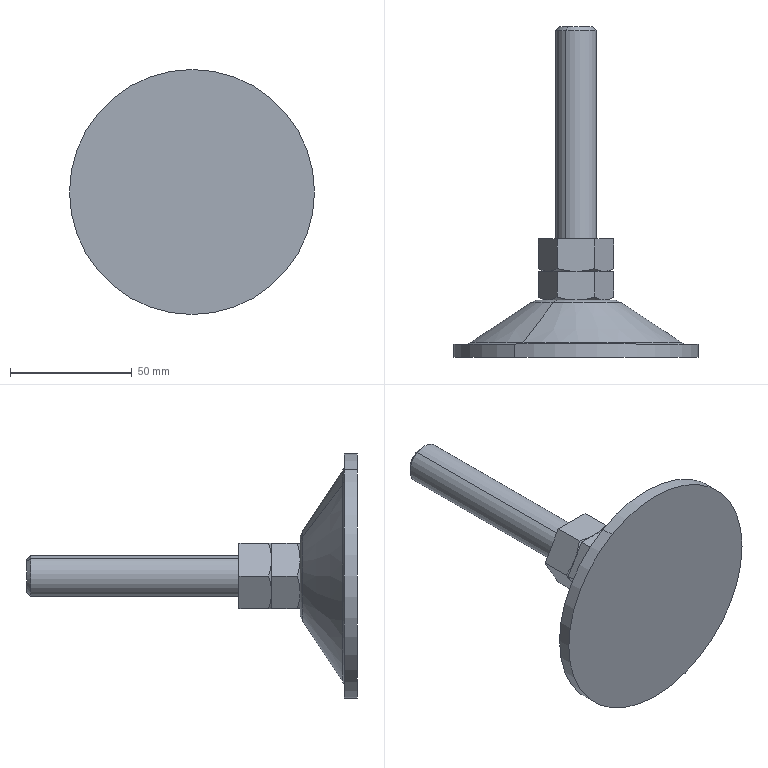Part | NX | 1 solid | 49 faces | box 100.8 x 136.08 x 100.8 mm | volume 135475 mm3 | plane 23 | cone 18 | torus 4 | cylinder 4 | commonest cylinder face diameters 16.8 x2 100.8 x2
STEP:
#1=CARTESIAN_POINT('',(301.832,-799.299,602.793));
#2=VERTEX_POINT('',#1);
#3=CARTESIAN_POINT('',(296.913,-799.299,597.874));
#4=VERTEX_POINT('',#3);
#5=CARTESIAN_POINT('',(290.193,-799.299,609.513));
#6=DIRECTION('',(0.,1.,0.));
#7=DIRECTION('',(0.5,0.,-0.866));
#8=AXIS2_PLACEMENT_3D('',#5,#6,#7);
#9=CIRCLE('',#8,13.44);
#10=EDGE_CURVE('',#2,#4,#9,.T.);
#11=ORIENTED_EDGE('',*,*,#10,.T.);
#12=CARTESIAN_POINT('',(297.952,-798.099,596.073));
#13=VERTEX_POINT('',#12);
#14=CARTESIAN_POINT('',(296.913,-799.299,597.874));
#15=DIRECTION('',(0.433,0.5,-0.75));
#16=VECTOR('',#15,1.);
#17=LINE('',#14,#16);
#18=EDGE_CURVE('',#4,#13,#17,.T.);
#19=ORIENTED_EDGE('',*,*,#18,.T.);
#20=CARTESIAN_POINT('',(301.832,-799.299,602.793));
#21=CARTESIAN_POINT('',(300.508,-799.299,600.5));
#22=CARTESIAN_POINT('',(299.22,-798.83,598.269));
#23=CARTESIAN_POINT('',(297.952,-798.099,596.073));
#24=B_SPLINE_CURVE_WITH_KNOTS('',3,(#20,#21,#22,#23),.UNSPECIFIED.,.F.,.F.,(4,4),(0.,1.),.UNSPECIFIED.);
#25=EDGE_CURVE('',#2,#13,#24,.T.);
#26=ORIENTED_EDGE('',*,*,#25,.F.);
#27=EDGE_LOOP('',(#11,#19,#26));
#28=FACE_OUTER_BOUND('',#27,.T.);
#29=CARTESIAN_POINT('',(290.193,-799.299,609.513));
#30=DIRECTION('',(0.,1.,0.));
#31=DIRECTION('',(0.5,0.,-0.866));
#32=AXIS2_PLACEMENT_3D('',#29,#30,#31);
#33=CONICAL_SURFACE('',#32,13.44,60.);
#34=ADVANCED_FACE('',(#28),#33,.T.);
#35=CARTESIAN_POINT('',(296.913,-787.539,597.874));
#36=VERTEX_POINT('',#35);
#37=CARTESIAN_POINT('',(301.832,-787.539,602.793));
#38=VERTEX_POINT('',#37);
#39=CARTESIAN_POINT('',(290.193,-787.539,609.513));
#40=DIRECTION('',(0.,-1.,0.));
#41=DIRECTION('',(0.5,0.,-0.866));
#42=AXIS2_PLACEMENT_3D('',#39,#40,#41);
#43=CIRCLE('',#42,13.44);
#44=EDGE_CURVE('',#36,#38,#43,.T.);
#45=ORIENTED_EDGE('',*,*,#44,.F.);
#46=CARTESIAN_POINT('',(297.952,-786.339,596.073));
#47=VERTEX_POINT('',#46);
#48=CARTESIAN_POINT('',(296.913,-787.539,597.874));
#49=DIRECTION('',(0.433,0.5,-0.75));
#50=VECTOR('',#49,1.);
#51=LINE('',#48,#50);
#52=EDGE_CURVE('',#36,#47,#51,.T.);
#53=ORIENTED_EDGE('',*,*,#52,.T.);
#54=CARTESIAN_POINT('',(301.832,-787.539,602.793));
#55=CARTESIAN_POINT('',(300.508,-787.539,600.5));
#56=CARTESIAN_POINT('',(299.22,-787.07,598.269));
#57=CARTESIAN_POINT('',(297.952,-786.339,596.073));
#58=B_SPLINE_CURVE_WITH_KNOTS('',3,(#54,#55,#56,#57),.UNSPECIFIED.,.F.,.F.,(4,4),(0.,1.),.UNSPECIFIED.);
#59=EDGE_CURVE('',#38,#47,#58,.T.);
#60=ORIENTED_EDGE('',*,*,#59,.F.);
#61=EDGE_LOOP('',(#45,#53,#60));
#62=FACE_OUTER_BOUND('',#61,.T.);
#63=CARTESIAN_POINT('',(290.193,-787.539,609.513));
#64=DIRECTION('',(0.,1.,0.));
#65=DIRECTION('',(0.5,0.,-0.866));
#66=AXIS2_PLACEMENT_3D('',#63,#64,#65);
#67=CONICAL_SURFACE('',#66,13.44,60.);
#68=ADVANCED_FACE('',(#62),#67,.T.);
#69=CARTESIAN_POINT('',(297.717,-799.299,596.481));
#70=VERTEX_POINT('',#69);
#71=CARTESIAN_POINT('',(282.668,-799.299,622.546));
#72=VERTEX_POINT('',#71);
#73=CARTESIAN_POINT('',(290.193,-799.299,609.513));
#74=DIRECTION('',(0.,1.,0.));
#75=DIRECTION('',(-0.5,0.,0.866));
#76=AXIS2_PLACEMENT_3D('',#73,#74,#75);
#77=CIRCLE('',#76,15.049);
#78=EDGE_CURVE('',#70,#72,#77,.T.);
#79=ORIENTED_EDGE('',*,*,#78,.F.);
#80=CARTESIAN_POINT('',(299.572,-800.415,593.269));
#81=VERTEX_POINT('',#80);
#82=CARTESIAN_POINT('',(297.717,-806.019,596.481));
#83=DIRECTION('',(-0.866,0.,-0.5));
#84=DIRECTION('',(-0.5,0.,0.866));
#85=AXIS2_PLACEMENT_3D('',#82,#83,#84);
#86=CIRCLE('',#85,6.72);
#87=EDGE_CURVE('',#70,#81,#86,.T.);
#88=ORIENTED_EDGE('',*,*,#87,.T.);
#89=CARTESIAN_POINT('',(280.814,-800.415,625.758));
#90=VERTEX_POINT('',#89);
#91=CARTESIAN_POINT('',(290.193,-800.415,609.513));
#92=DIRECTION('',(0.,1.,0.));
#93=DIRECTION('',(0.5,0.,-0.866));
#94=AXIS2_PLACEMENT_3D('',#91,#92,#93);
#95=CIRCLE('',#94,18.758);
#96=EDGE_CURVE('',#81,#90,#95,.T.);
#97=ORIENTED_EDGE('',*,*,#96,.T.);
#98=CARTESIAN_POINT('',(282.668,-806.019,622.546));
#99=DIRECTION('',(-0.866,0.,-0.5));
#100=DIRECTION('',(0.5,0.,-0.866));
#101=AXIS2_PLACEMENT_3D('',#98,#99,#100);
#102=CIRCLE('',#101,6.72);
#103=EDGE_CURVE('',#90,#72,#102,.T.);
#104=ORIENTED_EDGE('',*,*,#103,.T.);
#105=EDGE_LOOP('',(#79,#88,#97,#104));
#106=FACE_OUTER_BOUND('',#105,.T.);
#107=CARTESIAN_POINT('',(290.193,-806.019,609.513));
#108=DIRECTION('',(0.,-1.,0.));
#109=DIRECTION('',(-0.5,0.,0.866));
#110=AXIS2_PLACEMENT_3D('',#107,#108,#109);
#111=TOROIDAL_SURFACE('',#110,15.049,6.72);
#112=ADVANCED_FACE('',(#106),#111,.T.);
#113=CARTESIAN_POINT('',(285.993,-688.387,616.788));
#114=VERTEX_POINT('',#113);
#115=CARTESIAN_POINT('',(294.393,-688.387,602.239));
#116=VERTEX_POINT('',#115);
#117=CARTESIAN_POINT('',(290.193,-688.387,609.513));
#118=DIRECTION('',(0.,-1.,0.));
#119=DIRECTION('',(-0.5,0.,0.866));
#120=AXIS2_PLACEMENT_3D('',#117,#118,#119);
#121=CIRCLE('',#120,8.4);
#122=EDGE_CURVE('',#114,#116,#121,.T.);
#123=ORIENTED_EDGE('',*,*,#122,.T.);
#124=CARTESIAN_POINT('',(294.393,-774.099,602.239));
#125=VERTEX_POINT('',#124);
#126=CARTESIAN_POINT('',(294.393,-688.387,602.239));
#127=DIRECTION('',(0.,1.,0.));
#128=VECTOR('',#127,1.);
#129=LINE('',#126,#128);
#130=EDGE_CURVE('',#125,#116,#129,.T.);
#131=ORIENTED_EDGE('',*,*,#130,.F.);
#132=CARTESIAN_POINT('',(285.993,-774.099,616.788));
#133=VERTEX_POINT('',#132);
#134=CARTESIAN_POINT('',(290.193,-774.099,609.513));
#135=DIRECTION('',(0.,-1.,0.));
#136=DIRECTION('',(-0.5,0.,0.866));
#137=AXIS2_PLACEMENT_3D('',#134,#135,#136);
#138=CIRCLE('',#137,8.4);
#139=EDGE_CURVE('',#133,#125,#138,.T.);
#140=ORIENTED_EDGE('',*,*,#139,.F.);
#141=CARTESIAN_POINT('',(285.993,-688.387,616.788));
#142=DIRECTION('',(0.,-1.,0.));
#143=VECTOR('',#142,1.);
#144=LINE('',#141,#143);
#145=EDGE_CURVE('',#114,#133,#144,.T.);
#146=ORIENTED_EDGE('',*,*,#145,.F.);
#147=EDGE_LOOP('',(#123,#131,#140,#146));
#148=FACE_OUTER_BOUND('',#147,.T.);
#149=CARTESIAN_POINT('',(290.193,-688.387,609.513));
#150=DIRECTION('',(0.,-1.,0.));
#151=DIRECTION('',(-0.5,0.,0.866));
#152=AXIS2_PLACEMENT_3D('',#149,#150,#151);
#153=CYLINDRICAL_SURFACE('',#152,8.4);
#154=ADVANCED_FACE('',(#148),#153,.T.);
#155=ORIENTED_EDGE('',*,*,#96,.F.);
#156=CARTESIAN_POINT('',(312.013,-816.885,571.72));
#157=VERTEX_POINT('',#156);
#158=CARTESIAN_POINT('',(299.572,-800.415,593.269));
#159=DIRECTION('',(-0.4169,0.5519,0.7222));
#160=VECTOR('',#159,1.);
#161=LINE('',#158,#160);
#162=EDGE_CURVE('',#157,#81,#161,.T.);
#163=ORIENTED_EDGE('',*,*,#162,.F.);
#164=CARTESIAN_POINT('',(268.372,-816.885,647.307));
#165=VERTEX_POINT('',#164);
#166=CARTESIAN_POINT('',(290.193,-816.885,609.513));
#167=DIRECTION('',(0.,1.,0.));
#168=DIRECTION('',(0.5,0.,-0.866));
#169=AXIS2_PLACEMENT_3D('',#166,#167,#168);
#170=CIRCLE('',#169,43.641);
#171=EDGE_CURVE('',#157,#165,#170,.T.);
#172=ORIENTED_EDGE('',*,*,#171,.T.);
#173=CARTESIAN_POINT('',(280.814,-800.415,625.758));
#174=DIRECTION('',(-0.4169,-0.5519,0.7222));
#175=VECTOR('',#174,1.);
#176=LINE('',#173,#175);
#177=EDGE_CURVE('',#90,#165,#176,.T.);
#178=ORIENTED_EDGE('',*,*,#177,.F.);
#179=EDGE_LOOP('',(#155,#163,#172,#178));
#180=FACE_OUTER_BOUND('',#179,.T.);
#181=CARTESIAN_POINT('',(290.193,-800.415,609.513));
#182=DIRECTION('',(0.,-1.,0.));
#183=DIRECTION('',(-0.5,0.,0.866));
#184=AXIS2_PLACEMENT_3D('',#181,#182,#183);
#185=CONICAL_SURFACE('',#184,18.758,56.5);
#186=ADVANCED_FACE('',(#180),#185,.T.);
#187=CARTESIAN_POINT('',(286.817,-686.739,615.361));
#188=VERTEX_POINT('',#187);
#189=CARTESIAN_POINT('',(293.569,-686.739,603.666));
#190=VERTEX_POINT('',#189);
#191=CARTESIAN_POINT('',(290.193,-686.739,609.513));
#192=DIRECTION('',(0.,-1.,0.));
#193=DIRECTION('',(-0.5,0.,0.866));
#194=AXIS2_PLACEMENT_3D('',#191,#192,#193);
#195=CIRCLE('',#194,6.752);
#196=EDGE_CURVE('',#188,#190,#195,.T.);
#197=ORIENTED_EDGE('',*,*,#196,.T.);
#198=CARTESIAN_POINT('',(293.569,-686.739,603.666));
#199=DIRECTION('',(0.3536,-0.7071,-0.6124));
#200=VECTOR('',#199,1.);
#201=LINE('',#198,#200);
#202=EDGE_CURVE('',#190,#116,#201,.T.);
#203=ORIENTED_EDGE('',*,*,#202,.T.);
#204=ORIENTED_EDGE('',*,*,#122,.F.);
#205=CARTESIAN_POINT('',(286.817,-686.739,615.361));
#206=DIRECTION('',(0.3536,0.7071,-0.6124));
#207=VECTOR('',#206,1.);
#208=LINE('',#205,#207);
#209=EDGE_CURVE('',#114,#188,#208,.T.);
#210=ORIENTED_EDGE('',*,*,#209,.T.);
#211=EDGE_LOOP('',(#197,#203,#204,#210));
#212=FACE_OUTER_BOUND('',#211,.T.);
#213=CARTESIAN_POINT('',(290.193,-686.739,609.513));
#214=DIRECTION('',(0.,-1.,0.));
#215=DIRECTION('',(-0.5,0.,0.866));
#216=AXIS2_PLACEMENT_3D('',#213,#214,#215);
#217=CONICAL_SURFACE('',#216,6.752,45.);
#218=ADVANCED_FACE('',(#212),#217,.T.);
#219=CARTESIAN_POINT('',(290.193,-816.885,609.513));
#220=DIRECTION('',(0.,1.,0.));
#221=DIRECTION('',(0.5,0.,-0.866));
#222=AXIS2_PLACEMENT_3D('',#219,#220,#221);
#223=CIRCLE('',#222,43.641);
#224=EDGE_CURVE('',#165,#157,#223,.T.);
#225=ORIENTED_EDGE('',*,*,#224,.F.);
#226=CARTESIAN_POINT('',(267.445,-817.443,648.913));
#227=VERTEX_POINT('',#226);
#228=CARTESIAN_POINT('',(267.445,-814.083,648.913));
#229=DIRECTION('',(-0.866,0.,-0.5));
#230=DIRECTION('',(-0.5,0.,0.866));
#231=AXIS2_PLACEMENT_3D('',#228,#229,#230);
#232=CIRCLE('',#231,3.36);
#233=EDGE_CURVE('',#165,#227,#232,.T.);
#234=ORIENTED_EDGE('',*,*,#233,.T.);
#235=CARTESIAN_POINT('',(312.94,-817.443,570.113));
#236=VERTEX_POINT('',#235);
#237=CARTESIAN_POINT('',(290.193,-817.443,609.513));
#238=DIRECTION('',(0.,1.,0.));
#239=DIRECTION('',(0.5,0.,-0.866));
#240=AXIS2_PLACEMENT_3D('',#237,#238,#239);
#241=CIRCLE('',#240,45.495);
#242=EDGE_CURVE('',#227,#236,#241,.T.);
#243=ORIENTED_EDGE('',*,*,#242,.T.);
#244=CARTESIAN_POINT('',(312.94,-814.083,570.113));
#245=DIRECTION('',(-0.866,0.,-0.5));
#246=DIRECTION('',(0.5,0.,-0.866));
#247=AXIS2_PLACEMENT_3D('',#244,#245,#246);
#248=CIRCLE('',#247,3.36);
#249=EDGE_CURVE('',#236,#157,#248,.T.);
#250=ORIENTED_EDGE('',*,*,#249,.T.);
#251=EDGE_LOOP('',(#225,#234,#243,#250));
#252=FACE_OUTER_BOUND('',#251,.T.);
#253=CARTESIAN_POINT('',(290.193,-814.083,609.513));
#254=DIRECTION('',(0.,1.,0.));
#255=DIRECTION('',(0.5,0.,-0.866));
#256=AXIS2_PLACEMENT_3D('',#253,#254,#255);
#257=TOROIDAL_SURFACE('',#256,45.495,3.36);
#258=ADVANCED_FACE('',(#252),#257,.F.);
#259=CARTESIAN_POINT('',(315.393,-817.443,565.866));
#260=VERTEX_POINT('',#259);
#261=CARTESIAN_POINT('',(264.993,-817.443,653.161));
#262=VERTEX_POINT('',#261);
#263=CARTESIAN_POINT('',(290.193,-817.443,609.513));
#264=DIRECTION('',(0.,1.,0.));
#265=DIRECTION('',(-0.5,0.,0.866));
#266=AXIS2_PLACEMENT_3D('',#263,#264,#265);
#267=CIRCLE('',#266,50.4);
#268=EDGE_CURVE('',#260,#262,#267,.T.);
#269=ORIENTED_EDGE('',*,*,#268,.F.);
#270=CARTESIAN_POINT('',(315.393,-822.819,565.866));
#271=VERTEX_POINT('',#270);
#272=CARTESIAN_POINT('',(315.393,-817.443,565.866));
#273=DIRECTION('',(0.,-1.,0.));
#274=VECTOR('',#273,1.);
#275=LINE('',#272,#274);
#276=EDGE_CURVE('',#260,#271,#275,.T.);
#277=ORIENTED_EDGE('',*,*,#276,.T.);
#278=CARTESIAN_POINT('',(264.993,-822.819,653.161));
#279=VERTEX_POINT('',#278);
#280=CARTESIAN_POINT('',(290.193,-822.819,609.513));
#281=DIRECTION('',(0.,1.,0.));
#282=DIRECTION('',(-0.5,0.,0.866));
#283=AXIS2_PLACEMENT_3D('',#280,#281,#282);
#284=CIRCLE('',#283,50.4);
#285=EDGE_CURVE('',#271,#279,#284,.T.);
#286=ORIENTED_EDGE('',*,*,#285,.T.);
#287=CARTESIAN_POINT('',(264.993,-817.443,653.161));
#288=DIRECTION('',(0.,1.,0.));
#289=VECTOR('',#288,1.);
#290=LINE('',#287,#289);
#291=EDGE_CURVE('',#279,#262,#290,.T.);
#292=ORIENTED_EDGE('',*,*,#291,.T.);
#293=EDGE_LOOP('',(#269,#277,#286,#292));
#294=FACE_OUTER_BOUND('',#293,.T.);
#295=CARTESIAN_POINT('',(290.193,-817.443,609.513));
#296=DIRECTION('',(0.,-1.,0.));
#297=DIRECTION('',(-0.5,0.,0.866));
#298=AXIS2_PLACEMENT_3D('',#295,#296,#297);
#299=CYLINDRICAL_SURFACE('',#298,50.4);
#300=ADVANCED_FACE('',(#294),#299,.T.);
#301=CARTESIAN_POINT('',(301.832,-787.539,616.233));
#302=VERTEX_POINT('',#301);
#303=CARTESIAN_POINT('',(305.712,-786.339,609.513));
#304=VERTEX_POINT('',#303);
#305=CARTESIAN_POINT('',(301.832,-787.539,616.233));
#306=CARTESIAN_POINT('',(303.156,-787.539,613.94));
#307=CARTESIAN_POINT('',(304.444,-787.07,611.709));
#308=CARTESIAN_POINT('',(305.712,-786.339,609.513));
#309=B_SPLINE_CURVE_WITH_KNOTS('',3,(#305,#306,#307,#308),.UNSPECIFIED.,.F.,.F.,(4,4),(0.,1.),.UNSPECIFIED.);
#310=EDGE_CURVE('',#302,#304,#309,.T.);
#311=ORIENTED_EDGE('',*,*,#310,.F.);
#312=CARTESIAN_POINT('',(290.193,-787.539,609.513));
#313=DIRECTION('',(0.,1.,0.));
#314=DIRECTION('',(0.5,0.,-0.866));
#315=AXIS2_PLACEMENT_3D('',#312,#313,#314);
#316=CIRCLE('',#315,13.44);
#317=EDGE_CURVE('',#302,#38,#316,.T.);
#318=ORIENTED_EDGE('',*,*,#317,.T.);
#319=CARTESIAN_POINT('',(301.832,-787.539,602.793));
#320=CARTESIAN_POINT('',(303.156,-787.539,605.087));
#321=CARTESIAN_POINT('',(304.444,-787.07,607.318));
#322=CARTESIAN_POINT('',(305.712,-786.339,609.513));
#323=B_SPLINE_CURVE_WITH_KNOTS('',3,(#319,#320,#321,#322),.UNSPECIFIED.,.F.,.F.,(4,4),(0.,1.),.UNSPECIFIED.);
#324=EDGE_CURVE('',#38,#304,#323,.T.);
#325=ORIENTED_EDGE('',*,*,#324,.T.);
#326=EDGE_LOOP('',(#311,#318,#325));
#327=FACE_OUTER_BOUND('',#326,.T.);
#328=CARTESIAN_POINT('',(290.193,-787.539,609.513));
#329=DIRECTION('',(0.,1.,0.));
#330=DIRECTION('',(0.5,0.,-0.866));
#331=AXIS2_PLACEMENT_3D('',#328,#329,#330);
#332=CONICAL_SURFACE('',#331,13.44,60.);
#333=ADVANCED_FACE('',(#327),#332,.T.);
#334=CARTESIAN_POINT('',(305.712,-787.539,609.513));
#335=VERTEX_POINT('',#334);
#336=CARTESIAN_POINT('',(304.742,-787.539,611.193));
#337=DIRECTION('',(0.5,0.,-0.866));
#338=VECTOR('',#337,1.);
#339=LINE('',#336,#338);
#340=EDGE_CURVE('',#302,#335,#339,.T.);
#341=ORIENTED_EDGE('',*,*,#340,.T.);
#342=CARTESIAN_POINT('',(305.712,-787.539,609.513));
#343=DIRECTION('',(-0.5,0.,-0.866));
#344=VECTOR('',#343,1.);
#345=LINE('',#342,#344);
#346=EDGE_CURVE('',#335,#38,#345,.T.);
#347=ORIENTED_EDGE('',*,*,#346,.T.);
#348=ORIENTED_EDGE('',*,*,#317,.F.);
#349=EDGE_LOOP('',(#341,#347,#348));
#350=FACE_OUTER_BOUND('',#349,.T.);
#351=CARTESIAN_POINT('',(301.832,-787.539,616.233));
#352=DIRECTION('',(0.,1.,0.));
#353=DIRECTION('',(0.5,0.,-0.866));
#354=AXIS2_PLACEMENT_3D('',#351,#352,#353);
#355=PLANE('',#354);
#356=ADVANCED_FACE('',(#350),#355,.T.);
#357=CARTESIAN_POINT('',(305.712,-798.099,609.513));
#358=VERTEX_POINT('',#357);
#359=CARTESIAN_POINT('',(305.712,-793.419,609.513));
#360=DIRECTION('',(0.,-1.,0.));
#361=VECTOR('',#360,1.);
#362=LINE('',#359,#361);
#363=EDGE_CURVE('',#335,#358,#362,.T.);
#364=ORIENTED_EDGE('',*,*,#363,.T.);
#365=CARTESIAN_POINT('',(305.712,-798.099,609.513));
#366=CARTESIAN_POINT('',(304.444,-798.83,607.318));
#367=CARTESIAN_POINT('',(303.156,-799.299,605.087));
#368=CARTESIAN_POINT('',(301.832,-799.299,602.793));
#369=B_SPLINE_CURVE_WITH_KNOTS('',3,(#365,#366,#367,#368),.UNSPECIFIED.,.F.,.F.,(4,4),(0.,1.),.UNSPECIFIED.);
#370=EDGE_CURVE('',#358,#2,#369,.T.);
#371=ORIENTED_EDGE('',*,*,#370,.T.);
#372=ORIENTED_EDGE('',*,*,#25,.T.);
#373=CARTESIAN_POINT('',(297.952,-787.539,596.073));
#374=VERTEX_POINT('',#373);
#375=CARTESIAN_POINT('',(297.952,-793.419,596.073));
#376=DIRECTION('',(0.,1.,0.));
#377=VECTOR('',#376,1.);
#378=LINE('',#375,#377);
#379=EDGE_CURVE('',#13,#374,#378,.T.);
#380=ORIENTED_EDGE('',*,*,#379,.T.);
#381=CARTESIAN_POINT('',(301.832,-787.539,602.793));
#382=DIRECTION('',(0.5,0.,0.866));
#383=VECTOR('',#382,1.);
#384=LINE('',#381,#383);
#385=EDGE_CURVE('',#374,#38,#384,.T.);
#386=ORIENTED_EDGE('',*,*,#385,.T.);
#387=ORIENTED_EDGE('',*,*,#346,.F.);
#388=EDGE_LOOP('',(#364,#371,#372,#380,#386,#387));
#389=FACE_OUTER_BOUND('',#388,.T.);
#390=CARTESIAN_POINT('',(305.712,-787.539,609.513));
#391=DIRECTION('',(0.866,0.,-0.5));
#392=DIRECTION('',(0.,-1.,0.));
#393=AXIS2_PLACEMENT_3D('',#390,#391,#392);
#394=PLANE('',#393);
#395=ADVANCED_FACE('',(#389),#394,.T.);
#396=CARTESIAN_POINT('',(297.952,-787.539,622.953));
#397=VERTEX_POINT('',#396);
#398=CARTESIAN_POINT('',(301.832,-787.539,616.233));
#399=DIRECTION('',(-0.5,0.,0.866));
#400=VECTOR('',#399,1.);
#401=LINE('',#398,#400);
#402=EDGE_CURVE('',#302,#397,#401,.T.);
#403=ORIENTED_EDGE('',*,*,#402,.T.);
#404=CARTESIAN_POINT('',(297.952,-798.099,622.953));
#405=VERTEX_POINT('',#404);
#406=CARTESIAN_POINT('',(297.952,-793.419,622.953));
#407=DIRECTION('',(0.,-1.,0.));
#408=VECTOR('',#407,1.);
#409=LINE('',#406,#408);
#410=EDGE_CURVE('',#397,#405,#409,.T.);
#411=ORIENTED_EDGE('',*,*,#410,.T.);
#412=CARTESIAN_POINT('',(301.832,-799.299,616.233));
#413=VERTEX_POINT('',#412);
#414=CARTESIAN_POINT('',(297.952,-798.099,622.953));
#415=CARTESIAN_POINT('',(299.22,-798.83,620.758));
#416=CARTESIAN_POINT('',(300.508,-799.299,618.527));
#417=CARTESIAN_POINT('',(301.832,-799.299,616.233));
#418=B_SPLINE_CURVE_WITH_KNOTS('',3,(#414,#415,#416,#417),.UNSPECIFIED.,.F.,.F.,(4,4),(0.,1.),.UNSPECIFIED.);
#419=EDGE_CURVE('',#405,#413,#418,.T.);
#420=ORIENTED_EDGE('',*,*,#419,.T.);
#421=CARTESIAN_POINT('',(301.832,-799.299,616.233));
#422=CARTESIAN_POINT('',(303.156,-799.299,613.94));
#423=CARTESIAN_POINT('',(304.444,-798.83,611.709));
#424=CARTESIAN_POINT('',(305.712,-798.099,609.513));
#425=B_SPLINE_CURVE_WITH_KNOTS('',3,(#421,#422,#423,#424),.UNSPECIFIED.,.F.,.F.,(4,4),(0.,1.),.UNSPECIFIED.);
#426=EDGE_CURVE('',#413,#358,#425,.T.);
#427=ORIENTED_EDGE('',*,*,#426,.T.);
#428=ORIENTED_EDGE('',*,*,#363,.F.);
#429=ORIENTED_EDGE('',*,*,#340,.F.);
#430=EDGE_LOOP('',(#403,#411,#420,#427,#428,#429));
#431=FACE_OUTER_BOUND('',#430,.T.);
#432=CARTESIAN_POINT('',(297.952,-787.539,622.953));
#433=DIRECTION('',(0.866,0.,0.5));
#434=DIRECTION('',(0.,-1.,0.));
#435=AXIS2_PLACEMENT_3D('',#432,#433,#434);
#436=PLANE('',#435);
#437=ADVANCED_FACE('',(#431),#436,.T.);
#438=ORIENTED_EDGE('',*,*,#426,.F.);
#439=CARTESIAN_POINT('',(290.193,-799.299,609.513));
#440=DIRECTION('',(0.,1.,0.));
#441=DIRECTION('',(0.5,0.,-0.866));
#442=AXIS2_PLACEMENT_3D('',#439,#440,#441);
#443=CIRCLE('',#442,13.44);
#444=EDGE_CURVE('',#413,#2,#443,.T.);
#445=ORIENTED_EDGE('',*,*,#444,.T.);
#446=ORIENTED_EDGE('',*,*,#370,.F.);
#447=EDGE_LOOP('',(#438,#445,#446));
#448=FACE_OUTER_BOUND('',#447,.T.);
#449=CARTESIAN_POINT('',(290.193,-799.299,609.513));
#450=DIRECTION('',(0.,1.,0.));
#451=DIRECTION('',(0.5,0.,-0.866));
#452=AXIS2_PLACEMENT_3D('',#449,#450,#451);
#453=CONICAL_SURFACE('',#452,13.44,60.);
#454=ADVANCED_FACE('',(#448),#453,.T.);
#455=ORIENTED_EDGE('',*,*,#385,.F.);
#456=CARTESIAN_POINT('',(290.193,-787.539,596.073));
#457=VERTEX_POINT('',#456);
#458=CARTESIAN_POINT('',(297.952,-787.539,596.073));
#459=DIRECTION('',(-1.,0.,0.));
#460=VECTOR('',#459,1.);
#461=LINE('',#458,#460);
#462=EDGE_CURVE('',#374,#457,#461,.T.);
#463=ORIENTED_EDGE('',*,*,#462,.T.);
#464=CARTESIAN_POINT('',(290.193,-787.539,609.513));
#465=DIRECTION('',(0.,-1.,0.));
#466=DIRECTION('',(0.5,0.,-0.866));
#467=AXIS2_PLACEMENT_3D('',#464,#465,#466);
#468=CIRCLE('',#467,13.44);
#469=EDGE_CURVE('',#457,#36,#468,.T.);
#470=ORIENTED_EDGE('',*,*,#469,.T.);
#471=ORIENTED_EDGE('',*,*,#44,.T.);
#472=EDGE_LOOP('',(#455,#463,#470,#471));
#473=FACE_OUTER_BOUND('',#472,.T.);
#474=CARTESIAN_POINT('',(301.832,-787.539,602.793));
#475=DIRECTION('',(0.,1.,0.));
#476=DIRECTION('',(0.5,0.,-0.866));
#477=AXIS2_PLACEMENT_3D('',#474,#475,#476);
#478=PLANE('',#477);
#479=ADVANCED_FACE('',(#473),#478,.T.);
#480=ORIENTED_EDGE('',*,*,#379,.F.);
#481=CARTESIAN_POINT('',(290.193,-799.299,596.073));
#482=VERTEX_POINT('',#481);
#483=CARTESIAN_POINT('',(297.952,-798.099,596.073));
#484=CARTESIAN_POINT('',(295.417,-798.83,596.073));
#485=CARTESIAN_POINT('',(292.841,-799.299,596.073));
#486=CARTESIAN_POINT('',(290.193,-799.299,596.073));
#487=B_SPLINE_CURVE_WITH_KNOTS('',3,(#483,#484,#485,#486),.UNSPECIFIED.,.F.,.F.,(4,4),(0.,1.),.UNSPECIFIED.);
#488=EDGE_CURVE('',#13,#482,#487,.T.);
#489=ORIENTED_EDGE('',*,*,#488,.T.);
#490=CARTESIAN_POINT('',(282.433,-798.099,596.073));
#491=VERTEX_POINT('',#490);
#492=CARTESIAN_POINT('',(290.193,-799.299,596.073));
#493=CARTESIAN_POINT('',(287.544,-799.299,596.073));
#494=CARTESIAN_POINT('',(284.968,-798.83,596.073));
#495=CARTESIAN_POINT('',(282.433,-798.099,596.073));
#496=B_SPLINE_CURVE_WITH_KNOTS('',3,(#492,#493,#494,#495),.UNSPECIFIED.,.F.,.F.,(4,4),(0.,1.),.UNSPECIFIED.);
#497=EDGE_CURVE('',#482,#491,#496,.T.);
#498=ORIENTED_EDGE('',*,*,#497,.T.);
#499=CARTESIAN_POINT('',(282.433,-787.539,596.073));
#500=VERTEX_POINT('',#499);
#501=CARTESIAN_POINT('',(282.433,-793.419,596.073));
#502=DIRECTION('',(0.,1.,0.));
#503=VECTOR('',#502,1.);
#504=LINE('',#501,#503);
#505=EDGE_CURVE('',#491,#500,#504,.T.);
#506=ORIENTED_EDGE('',*,*,#505,.T.);
#507=CARTESIAN_POINT('',(290.193,-787.539,596.073));
#508=DIRECTION('',(1.,0.,0.));
#509=VECTOR('',#508,1.);
#510=LINE('',#507,#509);
#511=EDGE_CURVE('',#500,#457,#510,.T.);
#512=ORIENTED_EDGE('',*,*,#511,.T.);
#513=ORIENTED_EDGE('',*,*,#462,.F.);
#514=EDGE_LOOP('',(#480,#489,#498,#506,#512,#513));
#515=FACE_OUTER_BOUND('',#514,.T.);
#516=CARTESIAN_POINT('',(297.952,-787.539,596.073));
#517=DIRECTION('',(0.,0.,-1.));
#518=DIRECTION('',(0.,-1.,0.));
#519=AXIS2_PLACEMENT_3D('',#516,#517,#518);
#520=PLANE('',#519);
#521=ADVANCED_FACE('',(#515),#520,.T.);
#522=ORIENTED_EDGE('',*,*,#18,.F.);
#523=CARTESIAN_POINT('',(290.193,-799.299,609.513));
#524=DIRECTION('',(0.,1.,0.));
#525=DIRECTION('',(0.5,0.,-0.866));
#526=AXIS2_PLACEMENT_3D('',#523,#524,#525);
#527=CIRCLE('',#526,13.44);
#528=EDGE_CURVE('',#4,#482,#527,.T.);
#529=ORIENTED_EDGE('',*,*,#528,.T.);
#530=ORIENTED_EDGE('',*,*,#488,.F.);
#531=EDGE_LOOP('',(#522,#529,#530));
#532=FACE_OUTER_BOUND('',#531,.T.);
#533=CARTESIAN_POINT('',(290.193,-799.299,609.513));
#534=DIRECTION('',(0.,1.,0.));
#535=DIRECTION('',(0.5,0.,-0.866));
#536=AXIS2_PLACEMENT_3D('',#533,#534,#535);
#537=CONICAL_SURFACE('',#536,13.44,60.);
#538=ADVANCED_FACE('',(#532),#537,.T.);
#539=CARTESIAN_POINT('',(290.193,-787.539,622.953));
#540=VERTEX_POINT('',#539);
#541=CARTESIAN_POINT('',(282.433,-787.539,622.953));
#542=VERTEX_POINT('',#541);
#543=CARTESIAN_POINT('',(290.193,-787.539,622.953));
#544=DIRECTION('',(-1.,0.,0.));
#545=VECTOR('',#544,1.);
#546=LINE('',#543,#545);
#547=EDGE_CURVE('',#540,#542,#546,.T.);
#548=ORIENTED_EDGE('',*,*,#547,.T.);
#549=CARTESIAN_POINT('',(282.433,-798.099,622.953));
#550=VERTEX_POINT('',#549);
#551=CARTESIAN_POINT('',(282.433,-793.419,622.953));
#552=DIRECTION('',(0.,-1.,0.));
#553=VECTOR('',#552,1.);
#554=LINE('',#551,#553);
#555=EDGE_CURVE('',#542,#550,#554,.T.);
#556=ORIENTED_EDGE('',*,*,#555,.T.);
#557=CARTESIAN_POINT('',(290.193,-799.299,622.953));
#558=VERTEX_POINT('',#557);
#559=CARTESIAN_POINT('',(282.433,-798.099,622.953));
#560=CARTESIAN_POINT('',(284.968,-798.83,622.953));
#561=CARTESIAN_POINT('',(287.544,-799.299,622.953));
#562=CARTESIAN_POINT('',(290.193,-799.299,622.953));
#563=B_SPLINE_CURVE_WITH_KNOTS('',3,(#559,#560,#561,#562),.UNSPECIFIED.,.F.,.F.,(4,4),(0.,1.),.UNSPECIFIED.);
#564=EDGE_CURVE('',#550,#558,#563,.T.);
#565=ORIENTED_EDGE('',*,*,#564,.T.);
#566=CARTESIAN_POINT('',(290.193,-799.299,622.953));
#567=CARTESIAN_POINT('',(292.841,-799.299,622.953));
#568=CARTESIAN_POINT('',(295.417,-798.83,622.953));
#569=CARTESIAN_POINT('',(297.952,-798.099,622.953));
#570=B_SPLINE_CURVE_WITH_KNOTS('',3,(#566,#567,#568,#569),.UNSPECIFIED.,.F.,.F.,(4,4),(0.,1.),.UNSPECIFIED.);
#571=EDGE_CURVE('',#558,#405,#570,.T.);
#572=ORIENTED_EDGE('',*,*,#571,.T.);
#573=ORIENTED_EDGE('',*,*,#410,.F.);
#574=CARTESIAN_POINT('',(290.193,-787.539,622.953));
#575=DIRECTION('',(-1.,0.,0.));
#576=VECTOR('',#575,1.);
#577=LINE('',#574,#576);
#578=EDGE_CURVE('',#397,#540,#577,.T.);
#579=ORIENTED_EDGE('',*,*,#578,.T.);
#580=EDGE_LOOP('',(#548,#556,#565,#572,#573,#579));
#581=FACE_OUTER_BOUND('',#580,.T.);
#582=CARTESIAN_POINT('',(297.952,-799.299,622.953));
#583=DIRECTION('',(0.,0.,1.));
#584=DIRECTION('',(0.,1.,0.));
#585=AXIS2_PLACEMENT_3D('',#582,#583,#584);
#586=PLANE('',#585);
#587=ADVANCED_FACE('',(#581),#586,.T.);
#588=ORIENTED_EDGE('',*,*,#578,.F.);
#589=ORIENTED_EDGE('',*,*,#402,.F.);
#590=CARTESIAN_POINT('',(290.193,-787.539,609.513));
#591=DIRECTION('',(0.,-1.,0.));
#592=DIRECTION('',(0.5,0.,-0.866));
#593=AXIS2_PLACEMENT_3D('',#590,#591,#592);
#594=CIRCLE('',#593,13.44);
#595=EDGE_CURVE('',#302,#540,#594,.T.);
#596=ORIENTED_EDGE('',*,*,#595,.T.);
#597=EDGE_LOOP('',(#588,#589,#596));
#598=FACE_OUTER_BOUND('',#597,.T.);
#599=CARTESIAN_POINT('',(296.012,-787.539,626.313));
#600=DIRECTION('',(0.,1.,0.));
#601=DIRECTION('',(0.5,0.,-0.866));
#602=AXIS2_PLACEMENT_3D('',#599,#600,#601);
#603=PLANE('',#602);
#604=ADVANCED_FACE('',(#598),#603,.T.);
#605=CARTESIAN_POINT('',(290.193,-799.299,609.513));
#606=DIRECTION('',(0.,1.,0.));
#607=DIRECTION('',(0.5,0.,-0.866));
#608=AXIS2_PLACEMENT_3D('',#605,#606,#607);
#609=CIRCLE('',#608,13.44);
#610=EDGE_CURVE('',#558,#413,#609,.T.);
#611=ORIENTED_EDGE('',*,*,#610,.T.);
#612=ORIENTED_EDGE('',*,*,#419,.F.);
#613=ORIENTED_EDGE('',*,*,#571,.F.);
#614=EDGE_LOOP('',(#611,#612,#613));
#615=FACE_OUTER_BOUND('',#614,.T.);
#616=CARTESIAN_POINT('',(290.193,-799.299,609.513));
#617=DIRECTION('',(0.,1.,0.));
#618=DIRECTION('',(0.5,0.,-0.866));
#619=AXIS2_PLACEMENT_3D('',#616,#617,#618);
#620=CONICAL_SURFACE('',#619,13.44,60.);
#621=ADVANCED_FACE('',(#615),#620,.T.);
#622=CARTESIAN_POINT('',(297.952,-774.099,596.073));
#623=VERTEX_POINT('',#622);
#624=CARTESIAN_POINT('',(305.712,-774.099,609.513));
#625=VERTEX_POINT('',#624);
#626=CARTESIAN_POINT('',(301.832,-774.099,602.793));
#627=DIRECTION('',(0.5,0.,0.866));
#628=VECTOR('',#627,1.);
#629=LINE('',#626,#628);
#630=EDGE_CURVE('',#623,#625,#629,.T.);
#631=ORIENTED_EDGE('',*,*,#630,.T.);
#632=CARTESIAN_POINT('',(305.712,-780.819,609.513));
#633=DIRECTION('',(0.,-1.,0.));
#634=VECTOR('',#633,1.);
#635=LINE('',#632,#634);
#636=EDGE_CURVE('',#625,#304,#635,.T.);
#637=ORIENTED_EDGE('',*,*,#636,.T.);
#638=ORIENTED_EDGE('',*,*,#324,.F.);
#639=ORIENTED_EDGE('',*,*,#59,.T.);
#640=CARTESIAN_POINT('',(297.952,-780.819,596.073));
#641=DIRECTION('',(0.,1.,0.));
#642=VECTOR('',#641,1.);
#643=LINE('',#640,#642);
#644=EDGE_CURVE('',#47,#623,#643,.T.);
#645=ORIENTED_EDGE('',*,*,#644,.T.);
#646=EDGE_LOOP('',(#631,#637,#638,#639,#645));
#647=FACE_OUTER_BOUND('',#646,.T.);
#648=CARTESIAN_POINT('',(305.712,-774.099,609.513));
#649=DIRECTION('',(0.866,0.,-0.5));
#650=DIRECTION('',(0.,-1.,0.));
#651=AXIS2_PLACEMENT_3D('',#648,#649,#650);
#652=PLANE('',#651);
#653=ADVANCED_FACE('',(#647),#652,.T.);
#654=CARTESIAN_POINT('',(290.193,-799.299,609.513));
#655=DIRECTION('',(0.,1.,0.));
#656=DIRECTION('',(-0.5,0.,0.866));
#657=AXIS2_PLACEMENT_3D('',#654,#655,#656);
#658=CIRCLE('',#657,15.049);
#659=EDGE_CURVE('',#72,#70,#658,.T.);
#660=ORIENTED_EDGE('',*,*,#659,.T.);
#661=ORIENTED_EDGE('',*,*,#78,.T.);
#662=EDGE_LOOP('',(#660,#661));
#663=FACE_BOUND('',#662,.T.);
#664=CARTESIAN_POINT('',(278.553,-799.299,616.233));
#665=VERTEX_POINT('',#664);
#666=CARTESIAN_POINT('',(290.193,-799.299,609.513));
#667=DIRECTION('',(0.,-1.,0.));
#668=DIRECTION('',(0.5,0.,-0.866));
#669=AXIS2_PLACEMENT_3D('',#666,#667,#668);
#670=CIRCLE('',#669,13.44);
#671=EDGE_CURVE('',#558,#665,#670,.T.);
#672=ORIENTED_EDGE('',*,*,#671,.T.);
#673=CARTESIAN_POINT('',(278.553,-799.299,602.793));
#674=VERTEX_POINT('',#673);
#675=CARTESIAN_POINT('',(290.193,-799.299,609.513));
#676=DIRECTION('',(0.,-1.,0.));
#677=DIRECTION('',(0.5,0.,-0.866));
#678=AXIS2_PLACEMENT_3D('',#675,#676,#677);
#679=CIRCLE('',#678,13.44);
#680=EDGE_CURVE('',#665,#674,#679,.T.);
#681=ORIENTED_EDGE('',*,*,#680,.T.);
#682=CARTESIAN_POINT('',(290.193,-799.299,609.513));
#683=DIRECTION('',(0.,-1.,0.));
#684=DIRECTION('',(0.5,0.,-0.866));
#685=AXIS2_PLACEMENT_3D('',#682,#683,#684);
#686=CIRCLE('',#685,13.44);
#687=EDGE_CURVE('',#674,#482,#686,.T.);
#688=ORIENTED_EDGE('',*,*,#687,.T.);
#689=ORIENTED_EDGE('',*,*,#528,.F.);
#690=ORIENTED_EDGE('',*,*,#10,.F.);
#691=ORIENTED_EDGE('',*,*,#444,.F.);
#692=ORIENTED_EDGE('',*,*,#610,.F.);
#693=EDGE_LOOP('',(#672,#681,#688,#689,#690,#691,#692));
#694=FACE_BOUND('',#693,.T.);
#695=CARTESIAN_POINT('',(295.964,-799.299,630.222));
#696=DIRECTION('',(0.,1.,0.));
#697=DIRECTION('',(0.5,0.,-0.866));
#698=AXIS2_PLACEMENT_3D('',#695,#696,#697);
#699=PLANE('',#698);
#700=ADVANCED_FACE('',(#663,#694),#699,.T.);
#701=ORIENTED_EDGE('',*,*,#52,.F.);
#702=ORIENTED_EDGE('',*,*,#469,.F.);
#703=CARTESIAN_POINT('',(290.193,-787.539,596.073));
#704=CARTESIAN_POINT('',(292.841,-787.539,596.073));
#705=CARTESIAN_POINT('',(295.417,-787.07,596.073));
#706=CARTESIAN_POINT('',(297.952,-786.339,596.073));
#707=B_SPLINE_CURVE_WITH_KNOTS('',3,(#703,#704,#705,#706),.UNSPECIFIED.,.F.,.F.,(4,4),(0.,1.),.UNSPECIFIED.);
#708=EDGE_CURVE('',#457,#47,#707,.T.);
#709=ORIENTED_EDGE('',*,*,#708,.T.);
#710=EDGE_LOOP('',(#701,#702,#709));
#711=FACE_OUTER_BOUND('',#710,.T.);
#712=CARTESIAN_POINT('',(290.193,-787.539,609.513));
#713=DIRECTION('',(0.,1.,0.));
#714=DIRECTION('',(0.5,0.,-0.866));
#715=AXIS2_PLACEMENT_3D('',#712,#713,#714);
#716=CONICAL_SURFACE('',#715,13.44,60.);
#717=ADVANCED_FACE('',(#711),#716,.T.);
#718=ORIENTED_EDGE('',*,*,#511,.F.);
#719=CARTESIAN_POINT('',(278.553,-787.539,602.793));
#720=VERTEX_POINT('',#719);
#721=CARTESIAN_POINT('',(281.463,-787.539,597.753));
#722=DIRECTION('',(-0.5,0.,0.866));
#723=VECTOR('',#722,1.);
#724=LINE('',#721,#723);
#725=EDGE_CURVE('',#500,#720,#724,.T.);
#726=ORIENTED_EDGE('',*,*,#725,.T.);
#727=CARTESIAN_POINT('',(290.193,-787.539,609.513));
#728=DIRECTION('',(0.,-1.,0.));
#729=DIRECTION('',(0.5,0.,-0.866));
#730=AXIS2_PLACEMENT_3D('',#727,#728,#729);
#731=CIRCLE('',#730,13.44);
#732=EDGE_CURVE('',#720,#457,#731,.T.);
#733=ORIENTED_EDGE('',*,*,#732,.T.);
#734=EDGE_LOOP('',(#718,#726,#733));
#735=FACE_OUTER_BOUND('',#734,.T.);
#736=CARTESIAN_POINT('',(284.373,-787.539,606.153));
#737=DIRECTION('',(0.,1.,0.));
#738=DIRECTION('',(0.5,0.,-0.866));
#739=AXIS2_PLACEMENT_3D('',#736,#737,#738);
#740=PLANE('',#739);
#741=ADVANCED_FACE('',(#735),#740,.T.);
#742=ORIENTED_EDGE('',*,*,#505,.F.);
#743=CARTESIAN_POINT('',(282.433,-798.099,596.073));
#744=CARTESIAN_POINT('',(281.165,-798.83,598.269));
#745=CARTESIAN_POINT('',(279.878,-799.299,600.5));
#746=CARTESIAN_POINT('',(278.553,-799.299,602.793));
#747=B_SPLINE_CURVE_WITH_KNOTS('',3,(#743,#744,#745,#746),.UNSPECIFIED.,.F.,.F.,(4,4),(0.,1.),.UNSPECIFIED.);
#748=EDGE_CURVE('',#491,#674,#747,.T.);
#749=ORIENTED_EDGE('',*,*,#748,.T.);
#750=CARTESIAN_POINT('',(274.674,-798.099,609.513));
#751=VERTEX_POINT('',#750);
#752=CARTESIAN_POINT('',(278.553,-799.299,602.793));
#753=CARTESIAN_POINT('',(277.229,-799.299,605.087));
#754=CARTESIAN_POINT('',(275.941,-798.83,607.318));
#755=CARTESIAN_POINT('',(274.674,-798.099,609.513));
#756=B_SPLINE_CURVE_WITH_KNOTS('',3,(#752,#753,#754,#755),.UNSPECIFIED.,.F.,.F.,(4,4),(0.,1.),.UNSPECIFIED.);
#757=EDGE_CURVE('',#674,#751,#756,.T.);
#758=ORIENTED_EDGE('',*,*,#757,.T.);
#759=CARTESIAN_POINT('',(274.674,-787.539,609.513));
#760=VERTEX_POINT('',#759);
#761=CARTESIAN_POINT('',(274.674,-793.419,609.513));
#762=DIRECTION('',(0.,1.,0.));
#763=VECTOR('',#762,1.);
#764=LINE('',#761,#763);
#765=EDGE_CURVE('',#751,#760,#764,.T.);
#766=ORIENTED_EDGE('',*,*,#765,.T.);
#767=CARTESIAN_POINT('',(278.553,-787.539,602.793));
#768=DIRECTION('',(0.5,0.,-0.866));
#769=VECTOR('',#768,1.);
#770=LINE('',#767,#769);
#771=EDGE_CURVE('',#760,#720,#770,.T.);
#772=ORIENTED_EDGE('',*,*,#771,.T.);
#773=ORIENTED_EDGE('',*,*,#725,.F.);
#774=EDGE_LOOP('',(#742,#749,#758,#766,#772,#773));
#775=FACE_OUTER_BOUND('',#774,.T.);
#776=CARTESIAN_POINT('',(274.674,-799.299,609.513));
#777=DIRECTION('',(-0.866,0.,-0.5));
#778=DIRECTION('',(0.,1.,0.));
#779=AXIS2_PLACEMENT_3D('',#776,#777,#778);
#780=PLANE('',#779);
#781=ADVANCED_FACE('',(#775),#780,.T.);
#782=ORIENTED_EDGE('',*,*,#497,.F.);
#783=ORIENTED_EDGE('',*,*,#687,.F.);
#784=ORIENTED_EDGE('',*,*,#748,.F.);
#785=EDGE_LOOP('',(#782,#783,#784));
#786=FACE_OUTER_BOUND('',#785,.T.);
#787=CARTESIAN_POINT('',(290.193,-799.299,609.513));
#788=DIRECTION('',(0.,1.,0.));
#789=DIRECTION('',(0.5,0.,-0.866));
#790=AXIS2_PLACEMENT_3D('',#787,#788,#789);
#791=CONICAL_SURFACE('',#790,13.44,60.);
#792=ADVANCED_FACE('',(#786),#791,.T.);
#793=CARTESIAN_POINT('',(278.553,-787.539,616.233));
#794=VERTEX_POINT('',#793);
#795=CARTESIAN_POINT('',(278.553,-787.539,616.233));
#796=DIRECTION('',(-0.5,0.,-0.866));
#797=VECTOR('',#796,1.);
#798=LINE('',#795,#797);
#799=EDGE_CURVE('',#794,#760,#798,.T.);
#800=ORIENTED_EDGE('',*,*,#799,.T.);
#801=ORIENTED_EDGE('',*,*,#765,.F.);
#802=CARTESIAN_POINT('',(274.674,-798.099,609.513));
#803=CARTESIAN_POINT('',(275.941,-798.83,611.709));
#804=CARTESIAN_POINT('',(277.229,-799.299,613.94));
#805=CARTESIAN_POINT('',(278.553,-799.299,616.233));
#806=B_SPLINE_CURVE_WITH_KNOTS('',3,(#802,#803,#804,#805),.UNSPECIFIED.,.F.,.F.,(4,4),(0.,1.),.UNSPECIFIED.);
#807=EDGE_CURVE('',#751,#665,#806,.T.);
#808=ORIENTED_EDGE('',*,*,#807,.T.);
#809=CARTESIAN_POINT('',(278.553,-799.299,616.233));
#810=CARTESIAN_POINT('',(279.878,-799.299,618.527));
#811=CARTESIAN_POINT('',(281.165,-798.83,620.758));
#812=CARTESIAN_POINT('',(282.433,-798.099,622.953));
#813=B_SPLINE_CURVE_WITH_KNOTS('',3,(#809,#810,#811,#812),.UNSPECIFIED.,.F.,.F.,(4,4),(0.,1.),.UNSPECIFIED.);
#814=EDGE_CURVE('',#665,#550,#813,.T.);
#815=ORIENTED_EDGE('',*,*,#814,.T.);
#816=ORIENTED_EDGE('',*,*,#555,.F.);
#817=CARTESIAN_POINT('',(278.553,-787.539,616.233));
#818=DIRECTION('',(-0.5,0.,-0.866));
#819=VECTOR('',#818,1.);
#820=LINE('',#817,#819);
#821=EDGE_CURVE('',#542,#794,#820,.T.);
#822=ORIENTED_EDGE('',*,*,#821,.T.);
#823=EDGE_LOOP('',(#800,#801,#808,#815,#816,#822));
#824=FACE_OUTER_BOUND('',#823,.T.);
#825=CARTESIAN_POINT('',(282.433,-799.299,622.953));
#826=DIRECTION('',(-0.866,0.,0.5));
#827=DIRECTION('',(0.,1.,0.));
#828=AXIS2_PLACEMENT_3D('',#825,#826,#827);
#829=PLANE('',#828);
#830=ADVANCED_FACE('',(#824),#829,.T.);
#831=ORIENTED_EDGE('',*,*,#821,.F.);
#832=ORIENTED_EDGE('',*,*,#547,.F.);
#833=CARTESIAN_POINT('',(290.193,-787.539,609.513));
#834=DIRECTION('',(0.,-1.,0.));
#835=DIRECTION('',(0.5,0.,-0.866));
#836=AXIS2_PLACEMENT_3D('',#833,#834,#835);
#837=CIRCLE('',#836,13.44);
#838=EDGE_CURVE('',#540,#794,#837,.T.);
#839=ORIENTED_EDGE('',*,*,#838,.T.);
#840=EDGE_LOOP('',(#831,#832,#839));
#841=FACE_OUTER_BOUND('',#840,.T.);
#842=CARTESIAN_POINT('',(288.253,-787.539,626.313));
#843=DIRECTION('',(0.,1.,0.));
#844=DIRECTION('',(0.5,0.,-0.866));
#845=AXIS2_PLACEMENT_3D('',#842,#843,#844);
#846=PLANE('',#845);
#847=ADVANCED_FACE('',(#841),#846,.T.);
#848=ORIENTED_EDGE('',*,*,#564,.F.);
#849=ORIENTED_EDGE('',*,*,#814,.F.);
#850=ORIENTED_EDGE('',*,*,#671,.F.);
#851=EDGE_LOOP('',(#848,#849,#850));
#852=FACE_OUTER_BOUND('',#851,.T.);
#853=CARTESIAN_POINT('',(290.193,-799.299,609.513));
#854=DIRECTION('',(0.,1.,0.));
#855=DIRECTION('',(0.5,0.,-0.866));
#856=AXIS2_PLACEMENT_3D('',#853,#854,#855);
#857=CONICAL_SURFACE('',#856,13.44,60.);
#858=ADVANCED_FACE('',(#852),#857,.T.);
#859=ORIENTED_EDGE('',*,*,#595,.F.);
#860=CARTESIAN_POINT('',(297.952,-786.339,622.953));
#861=VERTEX_POINT('',#860);
#862=CARTESIAN_POINT('',(301.832,-787.539,616.233));
#863=CARTESIAN_POINT('',(300.508,-787.539,618.527));
#864=CARTESIAN_POINT('',(299.22,-787.07,620.758));
#865=CARTESIAN_POINT('',(297.952,-786.339,622.953));
#866=B_SPLINE_CURVE_WITH_KNOTS('',3,(#862,#863,#864,#865),.UNSPECIFIED.,.F.,.F.,(4,4),(0.,1.),.UNSPECIFIED.);
#867=EDGE_CURVE('',#302,#861,#866,.T.);
#868=ORIENTED_EDGE('',*,*,#867,.T.);
#869=CARTESIAN_POINT('',(297.952,-786.339,622.953));
#870=CARTESIAN_POINT('',(295.417,-787.07,622.953));
#871=CARTESIAN_POINT('',(292.841,-787.539,622.953));
#872=CARTESIAN_POINT('',(290.193,-787.539,622.953));
#873=B_SPLINE_CURVE_WITH_KNOTS('',3,(#869,#870,#871,#872),.UNSPECIFIED.,.F.,.F.,(4,4),(0.,1.),.UNSPECIFIED.);
#874=EDGE_CURVE('',#861,#540,#873,.T.);
#875=ORIENTED_EDGE('',*,*,#874,.T.);
#876=EDGE_LOOP('',(#859,#868,#875));
#877=FACE_OUTER_BOUND('',#876,.T.);
#878=CARTESIAN_POINT('',(290.193,-787.539,609.513));
#879=DIRECTION('',(0.,1.,0.));
#880=DIRECTION('',(0.5,0.,-0.866));
#881=AXIS2_PLACEMENT_3D('',#878,#879,#880);
#882=CONICAL_SURFACE('',#881,13.44,60.);
#883=ADVANCED_FACE('',(#877),#882,.T.);
#884=CARTESIAN_POINT('',(297.952,-774.099,622.953));
#885=VERTEX_POINT('',#884);
#886=CARTESIAN_POINT('',(301.832,-774.099,616.233));
#887=DIRECTION('',(-0.5,0.,0.866));
#888=VECTOR('',#887,1.);
#889=LINE('',#886,#888);
#890=EDGE_CURVE('',#625,#885,#889,.T.);
#891=ORIENTED_EDGE('',*,*,#890,.T.);
#892=CARTESIAN_POINT('',(297.952,-780.819,622.953));
#893=DIRECTION('',(0.,-1.,0.));
#894=VECTOR('',#893,1.);
#895=LINE('',#892,#894);
#896=EDGE_CURVE('',#885,#861,#895,.T.);
#897=ORIENTED_EDGE('',*,*,#896,.T.);
#898=ORIENTED_EDGE('',*,*,#867,.F.);
#899=ORIENTED_EDGE('',*,*,#310,.T.);
#900=ORIENTED_EDGE('',*,*,#636,.F.);
#901=EDGE_LOOP('',(#891,#897,#898,#899,#900));
#902=FACE_OUTER_BOUND('',#901,.T.);
#903=CARTESIAN_POINT('',(297.952,-774.099,622.953));
#904=DIRECTION('',(0.866,0.,0.5));
#905=DIRECTION('',(0.,-1.,0.));
#906=AXIS2_PLACEMENT_3D('',#903,#904,#905);
#907=PLANE('',#906);
#908=ADVANCED_FACE('',(#902),#907,.T.);
#909=CARTESIAN_POINT('',(274.674,-774.099,609.513));
#910=VERTEX_POINT('',#909);
#911=CARTESIAN_POINT('',(282.433,-774.099,622.953));
#912=VERTEX_POINT('',#911);
#913=CARTESIAN_POINT('',(274.674,-774.099,609.513));
#914=DIRECTION('',(0.5,0.,0.866));
#915=VECTOR('',#914,1.);
#916=LINE('',#913,#915);
#917=EDGE_CURVE('',#910,#912,#916,.T.);
#918=ORIENTED_EDGE('',*,*,#917,.T.);
#919=CARTESIAN_POINT('',(282.433,-774.099,622.953));
#920=DIRECTION('',(1.,0.,0.));
#921=VECTOR('',#920,1.);
#922=LINE('',#919,#921);
#923=EDGE_CURVE('',#912,#885,#922,.T.);
#924=ORIENTED_EDGE('',*,*,#923,.T.);
#925=ORIENTED_EDGE('',*,*,#890,.F.);
#926=ORIENTED_EDGE('',*,*,#630,.F.);
#927=CARTESIAN_POINT('',(282.433,-774.099,596.073));
#928=VERTEX_POINT('',#927);
#929=CARTESIAN_POINT('',(297.952,-774.099,596.073));
#930=DIRECTION('',(-1.,0.,0.));
#931=VECTOR('',#930,1.);
#932=LINE('',#929,#931);
#933=EDGE_CURVE('',#623,#928,#932,.T.);
#934=ORIENTED_EDGE('',*,*,#933,.T.);
#935=CARTESIAN_POINT('',(278.553,-774.099,602.793));
#936=DIRECTION('',(-0.5,0.,0.866));
#937=VECTOR('',#936,1.);
#938=LINE('',#935,#937);
#939=EDGE_CURVE('',#928,#910,#938,.T.);
#940=ORIENTED_EDGE('',*,*,#939,.T.);
#941=EDGE_LOOP('',(#918,#924,#925,#926,#934,#940));
#942=FACE_BOUND('',#941,.T.);
#943=ORIENTED_EDGE('',*,*,#139,.T.);
#944=CARTESIAN_POINT('',(290.193,-774.099,609.513));
#945=DIRECTION('',(0.,-1.,0.));
#946=DIRECTION('',(-0.5,0.,0.866));
#947=AXIS2_PLACEMENT_3D('',#944,#945,#946);
#948=CIRCLE('',#947,8.4);
#949=EDGE_CURVE('',#125,#133,#948,.T.);
#950=ORIENTED_EDGE('',*,*,#949,.T.);
#951=EDGE_LOOP('',(#943,#950));
#952=FACE_BOUND('',#951,.T.);
#953=CARTESIAN_POINT('',(294.072,-774.099,629.673));
#954=DIRECTION('',(0.,1.,0.));
#955=DIRECTION('',(0.5,0.,-0.866));
#956=AXIS2_PLACEMENT_3D('',#953,#954,#955);
#957=PLANE('',#956);
#958=ADVANCED_FACE('',(#942,#952),#957,.T.);
#959=ORIENTED_EDGE('',*,*,#644,.F.);
#960=ORIENTED_EDGE('',*,*,#708,.F.);
#961=CARTESIAN_POINT('',(282.433,-786.339,596.073));
#962=VERTEX_POINT('',#961);
#963=CARTESIAN_POINT('',(290.193,-787.539,596.073));
#964=CARTESIAN_POINT('',(287.544,-787.539,596.073));
#965=CARTESIAN_POINT('',(284.968,-787.07,596.073));
#966=CARTESIAN_POINT('',(282.433,-786.339,596.073));
#967=B_SPLINE_CURVE_WITH_KNOTS('',3,(#963,#964,#965,#966),.UNSPECIFIED.,.F.,.F.,(4,4),(0.,1.),.UNSPECIFIED.);
#968=EDGE_CURVE('',#457,#962,#967,.T.);
#969=ORIENTED_EDGE('',*,*,#968,.T.);
#970=CARTESIAN_POINT('',(282.433,-780.819,596.073));
#971=DIRECTION('',(0.,1.,0.));
#972=VECTOR('',#971,1.);
#973=LINE('',#970,#972);
#974=EDGE_CURVE('',#962,#928,#973,.T.);
#975=ORIENTED_EDGE('',*,*,#974,.T.);
#976=ORIENTED_EDGE('',*,*,#933,.F.);
#977=EDGE_LOOP('',(#959,#960,#969,#975,#976));
#978=FACE_OUTER_BOUND('',#977,.T.);
#979=CARTESIAN_POINT('',(297.952,-774.099,596.073));
#980=DIRECTION('',(0.,0.,-1.));
#981=DIRECTION('',(0.,-1.,0.));
#982=AXIS2_PLACEMENT_3D('',#979,#980,#981);
#983=PLANE('',#982);
#984=ADVANCED_FACE('',(#978),#983,.T.);
#985=ORIENTED_EDGE('',*,*,#87,.F.);
#986=ORIENTED_EDGE('',*,*,#659,.F.);
#987=ORIENTED_EDGE('',*,*,#103,.F.);
#988=CARTESIAN_POINT('',(290.193,-800.415,609.513));
#989=DIRECTION('',(0.,1.,0.));
#990=DIRECTION('',(0.5,0.,-0.866));
#991=AXIS2_PLACEMENT_3D('',#988,#989,#990);
#992=CIRCLE('',#991,18.758);
#993=EDGE_CURVE('',#90,#81,#992,.T.);
#994=ORIENTED_EDGE('',*,*,#993,.T.);
#995=EDGE_LOOP('',(#985,#986,#987,#994));
#996=FACE_OUTER_BOUND('',#995,.T.);
#997=CARTESIAN_POINT('',(290.193,-806.019,609.513));
#998=DIRECTION('',(0.,-1.,0.));
#999=DIRECTION('',(-0.5,0.,0.866));
#1000=AXIS2_PLACEMENT_3D('',#997,#998,#999);
#1001=TOROIDAL_SURFACE('',#1000,15.049,6.72);
#1002=ADVANCED_FACE('',(#996),#1001,.T.);
#1003=ORIENTED_EDGE('',*,*,#680,.F.);
#1004=ORIENTED_EDGE('',*,*,#807,.F.);
#1005=ORIENTED_EDGE('',*,*,#757,.F.);
#1006=EDGE_LOOP('',(#1003,#1004,#1005));
#1007=FACE_OUTER_BOUND('',#1006,.T.);
#1008=CARTESIAN_POINT('',(290.193,-799.299,609.513));
#1009=DIRECTION('',(0.,1.,0.));
#1010=DIRECTION('',(0.5,0.,-0.866));
#1011=AXIS2_PLACEMENT_3D('',#1008,#1009,#1010);
#1012=CONICAL_SURFACE('',#1011,13.44,60.);
#1013=ADVANCED_FACE('',(#1007),#1012,.T.);
#1014=ORIENTED_EDGE('',*,*,#968,.F.);
#1015=ORIENTED_EDGE('',*,*,#732,.F.);
#1016=CARTESIAN_POINT('',(278.553,-787.539,602.793));
#1017=CARTESIAN_POINT('',(279.878,-787.539,600.5));
#1018=CARTESIAN_POINT('',(281.165,-787.07,598.269));
#1019=CARTESIAN_POINT('',(282.433,-786.339,596.073));
#1020=B_SPLINE_CURVE_WITH_KNOTS('',3,(#1016,#1017,#1018,#1019),.UNSPECIFIED.,.F.,.F.,(4,4),(0.,1.),.UNSPECIFIED.);
#1021=EDGE_CURVE('',#720,#962,#1020,.T.);
#1022=ORIENTED_EDGE('',*,*,#1021,.T.);
#1023=EDGE_LOOP('',(#1014,#1015,#1022));
#1024=FACE_OUTER_BOUND('',#1023,.T.);
#1025=CARTESIAN_POINT('',(290.193,-787.539,609.513));
#1026=DIRECTION('',(0.,1.,0.));
#1027=DIRECTION('',(0.5,0.,-0.866));
#1028=AXIS2_PLACEMENT_3D('',#1025,#1026,#1027);
#1029=CONICAL_SURFACE('',#1028,13.44,60.);
#1030=ADVANCED_FACE('',(#1024),#1029,.T.);
#1031=ORIENTED_EDGE('',*,*,#771,.F.);
#1032=ORIENTED_EDGE('',*,*,#799,.F.);
#1033=CARTESIAN_POINT('',(290.193,-787.539,609.513));
#1034=DIRECTION('',(0.,-1.,0.));
#1035=DIRECTION('',(0.5,0.,-0.866));
#1036=AXIS2_PLACEMENT_3D('',#1033,#1034,#1035);
#1037=CIRCLE('',#1036,13.44);
#1038=EDGE_CURVE('',#794,#720,#1037,.T.);
#1039=ORIENTED_EDGE('',*,*,#1038,.T.);
#1040=EDGE_LOOP('',(#1031,#1032,#1039));
#1041=FACE_OUTER_BOUND('',#1040,.T.);
#1042=CARTESIAN_POINT('',(278.553,-787.539,616.233));
#1043=DIRECTION('',(0.,1.,0.));
#1044=DIRECTION('',(0.5,0.,-0.866));
#1045=AXIS2_PLACEMENT_3D('',#1042,#1043,#1044);
#1046=PLANE('',#1045);
#1047=ADVANCED_FACE('',(#1041),#1046,.T.);
#1048=CARTESIAN_POINT('',(282.433,-786.339,622.953));
#1049=VERTEX_POINT('',#1048);
#1050=CARTESIAN_POINT('',(282.433,-786.339,622.953));
#1051=CARTESIAN_POINT('',(281.165,-787.07,620.758));
#1052=CARTESIAN_POINT('',(279.878,-787.539,618.527));
#1053=CARTESIAN_POINT('',(278.553,-787.539,616.233));
#1054=B_SPLINE_CURVE_WITH_KNOTS('',3,(#1050,#1051,#1052,#1053),.UNSPECIFIED.,.F.,.F.,(4,4),(0.,1.),.UNSPECIFIED.);
#1055=EDGE_CURVE('',#1049,#794,#1054,.T.);
#1056=ORIENTED_EDGE('',*,*,#1055,.T.);
#1057=ORIENTED_EDGE('',*,*,#838,.F.);
#1058=CARTESIAN_POINT('',(290.193,-787.539,622.953));
#1059=CARTESIAN_POINT('',(287.544,-787.539,622.953));
#1060=CARTESIAN_POINT('',(284.968,-787.07,622.953));
#1061=CARTESIAN_POINT('',(282.433,-786.339,622.953));
#1062=B_SPLINE_CURVE_WITH_KNOTS('',3,(#1058,#1059,#1060,#1061),.UNSPECIFIED.,.F.,.F.,(4,4),(0.,1.),.UNSPECIFIED.);
#1063=EDGE_CURVE('',#540,#1049,#1062,.T.);
#1064=ORIENTED_EDGE('',*,*,#1063,.T.);
#1065=EDGE_LOOP('',(#1056,#1057,#1064));
#1066=FACE_OUTER_BOUND('',#1065,.T.);
#1067=CARTESIAN_POINT('',(290.193,-787.539,609.513));
#1068=DIRECTION('',(0.,1.,0.));
#1069=DIRECTION('',(0.5,0.,-0.866));
#1070=AXIS2_PLACEMENT_3D('',#1067,#1068,#1069);
#1071=CONICAL_SURFACE('',#1070,13.44,60.);
#1072=ADVANCED_FACE('',(#1066),#1071,.T.);
#1073=ORIENTED_EDGE('',*,*,#923,.F.);
#1074=CARTESIAN_POINT('',(282.433,-780.819,622.953));
#1075=DIRECTION('',(0.,-1.,0.));
#1076=VECTOR('',#1075,1.);
#1077=LINE('',#1074,#1076);
#1078=EDGE_CURVE('',#912,#1049,#1077,.T.);
#1079=ORIENTED_EDGE('',*,*,#1078,.T.);
#1080=ORIENTED_EDGE('',*,*,#1063,.F.);
#1081=ORIENTED_EDGE('',*,*,#874,.F.);
#1082=ORIENTED_EDGE('',*,*,#896,.F.);
#1083=EDGE_LOOP('',(#1073,#1079,#1080,#1081,#1082));
#1084=FACE_OUTER_BOUND('',#1083,.T.);
#1085=CARTESIAN_POINT('',(297.952,-787.539,622.953));
#1086=DIRECTION('',(0.,0.,1.));
#1087=DIRECTION('',(0.,1.,0.));
#1088=AXIS2_PLACEMENT_3D('',#1085,#1086,#1087);
#1089=PLANE('',#1088);
#1090=ADVANCED_FACE('',(#1084),#1089,.T.);
#1091=CARTESIAN_POINT('',(274.674,-786.339,609.513));
#1092=VERTEX_POINT('',#1091);
#1093=CARTESIAN_POINT('',(274.674,-780.819,609.513));
#1094=DIRECTION('',(0.,-1.,0.));
#1095=VECTOR('',#1094,1.);
#1096=LINE('',#1093,#1095);
#1097=EDGE_CURVE('',#910,#1092,#1096,.T.);
#1098=ORIENTED_EDGE('',*,*,#1097,.T.);
#1099=CARTESIAN_POINT('',(274.674,-786.339,609.513));
#1100=CARTESIAN_POINT('',(275.941,-787.07,611.709));
#1101=CARTESIAN_POINT('',(277.229,-787.539,613.94));
#1102=CARTESIAN_POINT('',(278.553,-787.539,616.233));
#1103=B_SPLINE_CURVE_WITH_KNOTS('',3,(#1099,#1100,#1101,#1102),.UNSPECIFIED.,.F.,.F.,(4,4),(0.,1.),.UNSPECIFIED.);
#1104=EDGE_CURVE('',#1092,#794,#1103,.T.);
#1105=ORIENTED_EDGE('',*,*,#1104,.T.);
#1106=ORIENTED_EDGE('',*,*,#1055,.F.);
#1107=ORIENTED_EDGE('',*,*,#1078,.F.);
#1108=ORIENTED_EDGE('',*,*,#917,.F.);
#1109=EDGE_LOOP('',(#1098,#1105,#1106,#1107,#1108));
#1110=FACE_OUTER_BOUND('',#1109,.T.);
#1111=CARTESIAN_POINT('',(282.433,-787.539,622.953));
#1112=DIRECTION('',(-0.866,0.,0.5));
#1113=DIRECTION('',(0.,1.,0.));
#1114=AXIS2_PLACEMENT_3D('',#1111,#1112,#1113);
#1115=PLANE('',#1114);
#1116=ADVANCED_FACE('',(#1110),#1115,.T.);
#1117=ORIENTED_EDGE('',*,*,#974,.F.);
#1118=ORIENTED_EDGE('',*,*,#1021,.F.);
#1119=CARTESIAN_POINT('',(278.553,-787.539,602.793));
#1120=CARTESIAN_POINT('',(277.229,-787.539,605.087));
#1121=CARTESIAN_POINT('',(275.941,-787.07,607.318));
#1122=CARTESIAN_POINT('',(274.674,-786.339,609.513));
#1123=B_SPLINE_CURVE_WITH_KNOTS('',3,(#1119,#1120,#1121,#1122),.UNSPECIFIED.,.F.,.F.,(4,4),(0.,1.),.UNSPECIFIED.);
#1124=EDGE_CURVE('',#720,#1092,#1123,.T.);
#1125=ORIENTED_EDGE('',*,*,#1124,.T.);
#1126=ORIENTED_EDGE('',*,*,#1097,.F.);
#1127=ORIENTED_EDGE('',*,*,#939,.F.);
#1128=EDGE_LOOP('',(#1117,#1118,#1125,#1126,#1127));
#1129=FACE_OUTER_BOUND('',#1128,.T.);
#1130=CARTESIAN_POINT('',(274.674,-787.539,609.513));
#1131=DIRECTION('',(-0.866,0.,-0.5));
#1132=DIRECTION('',(0.,1.,0.));
#1133=AXIS2_PLACEMENT_3D('',#1130,#1131,#1132);
#1134=PLANE('',#1133);
#1135=ADVANCED_FACE('',(#1129),#1134,.T.);
#1136=ORIENTED_EDGE('',*,*,#130,.T.);
#1137=CARTESIAN_POINT('',(290.193,-688.387,609.513));
#1138=DIRECTION('',(0.,-1.,0.));
#1139=DIRECTION('',(-0.5,0.,0.866));
#1140=AXIS2_PLACEMENT_3D('',#1137,#1138,#1139);
#1141=CIRCLE('',#1140,8.4);
#1142=EDGE_CURVE('',#116,#114,#1141,.T.);
#1143=ORIENTED_EDGE('',*,*,#1142,.T.);
#1144=ORIENTED_EDGE('',*,*,#145,.T.);
#1145=ORIENTED_EDGE('',*,*,#949,.F.);
#1146=EDGE_LOOP('',(#1136,#1143,#1144,#1145));
#1147=FACE_OUTER_BOUND('',#1146,.T.);
#1148=CARTESIAN_POINT('',(290.193,-688.387,609.513));
#1149=DIRECTION('',(0.,-1.,0.));
#1150=DIRECTION('',(-0.5,0.,0.866));
#1151=AXIS2_PLACEMENT_3D('',#1148,#1149,#1150);
#1152=CYLINDRICAL_SURFACE('',#1151,8.4);
#1153=ADVANCED_FACE('',(#1147),#1152,.T.);
#1154=ORIENTED_EDGE('',*,*,#162,.T.);
#1155=ORIENTED_EDGE('',*,*,#993,.F.);
#1156=ORIENTED_EDGE('',*,*,#177,.T.);
#1157=ORIENTED_EDGE('',*,*,#224,.T.);
#1158=EDGE_LOOP('',(#1154,#1155,#1156,#1157));
#1159=FACE_OUTER_BOUND('',#1158,.T.);
#1160=CARTESIAN_POINT('',(290.193,-800.415,609.513));
#1161=DIRECTION('',(0.,-1.,0.));
#1162=DIRECTION('',(-0.5,0.,0.866));
#1163=AXIS2_PLACEMENT_3D('',#1160,#1161,#1162);
#1164=CONICAL_SURFACE('',#1163,18.758,56.5);
#1165=ADVANCED_FACE('',(#1159),#1164,.T.);
#1166=ORIENTED_EDGE('',*,*,#1124,.F.);
#1167=ORIENTED_EDGE('',*,*,#1038,.F.);
#1168=ORIENTED_EDGE('',*,*,#1104,.F.);
#1169=EDGE_LOOP('',(#1166,#1167,#1168));
#1170=FACE_OUTER_BOUND('',#1169,.T.);
#1171=CARTESIAN_POINT('',(290.193,-787.539,609.513));
#1172=DIRECTION('',(0.,1.,0.));
#1173=DIRECTION('',(0.5,0.,-0.866));
#1174=AXIS2_PLACEMENT_3D('',#1171,#1172,#1173);
#1175=CONICAL_SURFACE('',#1174,13.44,60.);
#1176=ADVANCED_FACE('',(#1170),#1175,.T.);
#1177=ORIENTED_EDGE('',*,*,#202,.F.);
#1178=CARTESIAN_POINT('',(290.193,-686.739,609.513));
#1179=DIRECTION('',(0.,-1.,0.));
#1180=DIRECTION('',(-0.5,0.,0.866));
#1181=AXIS2_PLACEMENT_3D('',#1178,#1179,#1180);
#1182=CIRCLE('',#1181,6.752);
#1183=EDGE_CURVE('',#190,#188,#1182,.T.);
#1184=ORIENTED_EDGE('',*,*,#1183,.T.);
#1185=ORIENTED_EDGE('',*,*,#209,.F.);
#1186=ORIENTED_EDGE('',*,*,#1142,.F.);
#1187=EDGE_LOOP('',(#1177,#1184,#1185,#1186));
#1188=FACE_OUTER_BOUND('',#1187,.T.);
#1189=CARTESIAN_POINT('',(290.193,-686.739,609.513));
#1190=DIRECTION('',(0.,-1.,0.));
#1191=DIRECTION('',(-0.5,0.,0.866));
#1192=AXIS2_PLACEMENT_3D('',#1189,#1190,#1191);
#1193=CONICAL_SURFACE('',#1192,6.752,45.);
#1194=ADVANCED_FACE('',(#1188),#1193,.T.);
#1195=ORIENTED_EDGE('',*,*,#233,.F.);
#1196=ORIENTED_EDGE('',*,*,#171,.F.);
#1197=ORIENTED_EDGE('',*,*,#249,.F.);
#1198=CARTESIAN_POINT('',(290.193,-817.443,609.513));
#1199=DIRECTION('',(0.,1.,0.));
#1200=DIRECTION('',(0.5,0.,-0.866));
#1201=AXIS2_PLACEMENT_3D('',#1198,#1199,#1200);
#1202=CIRCLE('',#1201,45.495);
#1203=EDGE_CURVE('',#236,#227,#1202,.T.);
#1204=ORIENTED_EDGE('',*,*,#1203,.T.);
#1205=EDGE_LOOP('',(#1195,#1196,#1197,#1204));
#1206=FACE_OUTER_BOUND('',#1205,.T.);
#1207=CARTESIAN_POINT('',(290.193,-814.083,609.513));
#1208=DIRECTION('',(0.,1.,0.));
#1209=DIRECTION('',(0.5,0.,-0.866));
#1210=AXIS2_PLACEMENT_3D('',#1207,#1208,#1209);
#1211=TOROIDAL_SURFACE('',#1210,45.495,3.36);
#1212=ADVANCED_FACE('',(#1206),#1211,.F.);
#1213=ORIENTED_EDGE('',*,*,#196,.F.);
#1214=ORIENTED_EDGE('',*,*,#1183,.F.);
#1215=EDGE_LOOP('',(#1213,#1214));
#1216=FACE_OUTER_BOUND('',#1215,.T.);
#1217=CARTESIAN_POINT('',(287.604,-686.739,600.223));
#1218=DIRECTION('',(0.,1.,0.));
#1219=DIRECTION('',(-0.5,0.,0.866));
#1220=AXIS2_PLACEMENT_3D('',#1217,#1218,#1219);
#1221=PLANE('',#1220);
#1222=ADVANCED_FACE('',(#1216),#1221,.T.);
#1223=ORIENTED_EDGE('',*,*,#1203,.F.);
#1224=ORIENTED_EDGE('',*,*,#242,.F.);
#1225=EDGE_LOOP('',(#1223,#1224));
#1226=FACE_BOUND('',#1225,.T.);
#1227=CARTESIAN_POINT('',(290.193,-817.443,609.513));
#1228=DIRECTION('',(0.,1.,0.));
#1229=DIRECTION('',(-0.5,0.,0.866));
#1230=AXIS2_PLACEMENT_3D('',#1227,#1228,#1229);
#1231=CIRCLE('',#1230,50.4);
#1232=EDGE_CURVE('',#262,#260,#1231,.T.);
#1233=ORIENTED_EDGE('',*,*,#1232,.T.);
#1234=ORIENTED_EDGE('',*,*,#268,.T.);
#1235=EDGE_LOOP('',(#1233,#1234));
#1236=FACE_BOUND('',#1235,.T.);
#1237=CARTESIAN_POINT('',(309.513,-817.443,678.865));
#1238=DIRECTION('',(0.,1.,0.));
#1239=DIRECTION('',(0.5,0.,-0.866));
#1240=AXIS2_PLACEMENT_3D('',#1237,#1238,#1239);
#1241=PLANE('',#1240);
#1242=ADVANCED_FACE('',(#1226,#1236),#1241,.T.);
#1243=ORIENTED_EDGE('',*,*,#276,.F.);
#1244=ORIENTED_EDGE('',*,*,#1232,.F.);
#1245=ORIENTED_EDGE('',*,*,#291,.F.);
#1246=CARTESIAN_POINT('',(290.193,-822.819,609.513));
#1247=DIRECTION('',(0.,1.,0.));
#1248=DIRECTION('',(-0.5,0.,0.866));
#1249=AXIS2_PLACEMENT_3D('',#1246,#1247,#1248);
#1250=CIRCLE('',#1249,50.4);
#1251=EDGE_CURVE('',#279,#271,#1250,.T.);
#1252=ORIENTED_EDGE('',*,*,#1251,.T.);
#1253=EDGE_LOOP('',(#1243,#1244,#1245,#1252));
#1254=FACE_OUTER_BOUND('',#1253,.T.);
#1255=CARTESIAN_POINT('',(290.193,-817.443,609.513));
#1256=DIRECTION('',(0.,-1.,0.));
#1257=DIRECTION('',(-0.5,0.,0.866));
#1258=AXIS2_PLACEMENT_3D('',#1255,#1256,#1257);
#1259=CYLINDRICAL_SURFACE('',#1258,50.4);
#1260=ADVANCED_FACE('',(#1254),#1259,.T.);
#1261=ORIENTED_EDGE('',*,*,#1251,.F.);
#1262=ORIENTED_EDGE('',*,*,#285,.F.);
#1263=EDGE_LOOP('',(#1261,#1262));
#1264=FACE_OUTER_BOUND('',#1263,.T.);
#1265=CARTESIAN_POINT('',(359.913,-822.819,591.57));
#1266=DIRECTION('',(0.,-1.,0.));
#1267=DIRECTION('',(-0.5,0.,0.866));
#1268=AXIS2_PLACEMENT_3D('',#1265,#1266,#1267);
#1269=PLANE('',#1268);
#1270=ADVANCED_FACE('',(#1264),#1269,.T.);
#1271=CLOSED_SHELL('',(#34,#68,#112,#154,#186,#218,#258,#300,#333,#356,#395,#437,#454,#479,#521,#538,#587,#604,#621,#653,#700,#717,#741,#781,#792,#830,#847,#858,#883,#908,#958,#984,#1002,#1013,#1030,#1047,#1072,#1090,#1116,#1135,#1153,#1165,#1176,#1194,#1212,#1222,#1242,#1260,#1270));
#1272=MANIFOLD_SOLID_BREP('',#1271);
#1273=(LENGTH_UNIT()NAMED_UNIT(*)SI_UNIT(.MILLI.,.METRE.));
#1274=UNCERTAINTY_MEASURE_WITH_UNIT(LENGTH_MEASURE(0.0508),#1273,'','');
#1275=(NAMED_UNIT(*)PLANE_ANGLE_UNIT()SI_UNIT($,.RADIAN.));
#1276=PLANE_ANGLE_MEASURE_WITH_UNIT(PLANE_ANGLE_MEASURE(0.01745),#1275);
#1277=DIMENSIONAL_EXPONENTS(0.,0.,0.,0.,0.,0.,0.);
#1278=(CONVERSION_BASED_UNIT('DEGREE',#1276)NAMED_UNIT(#1277)PLANE_ANGLE_UNIT());
#1279=(NAMED_UNIT(*)SI_UNIT($,.STERADIAN.)SOLID_ANGLE_UNIT());
#1280=(GEOMETRIC_REPRESENTATION_CONTEXT(3)GLOBAL_UNCERTAINTY_ASSIGNED_CONTEXT((#1274))GLOBAL_UNIT_ASSIGNED_CONTEXT((#1273,#1278,#1279))REPRESENTATION_CONTEXT('',''));
#1281=ADVANCED_BREP_SHAPE_REPRESENTATION('',(#1272),#1280);